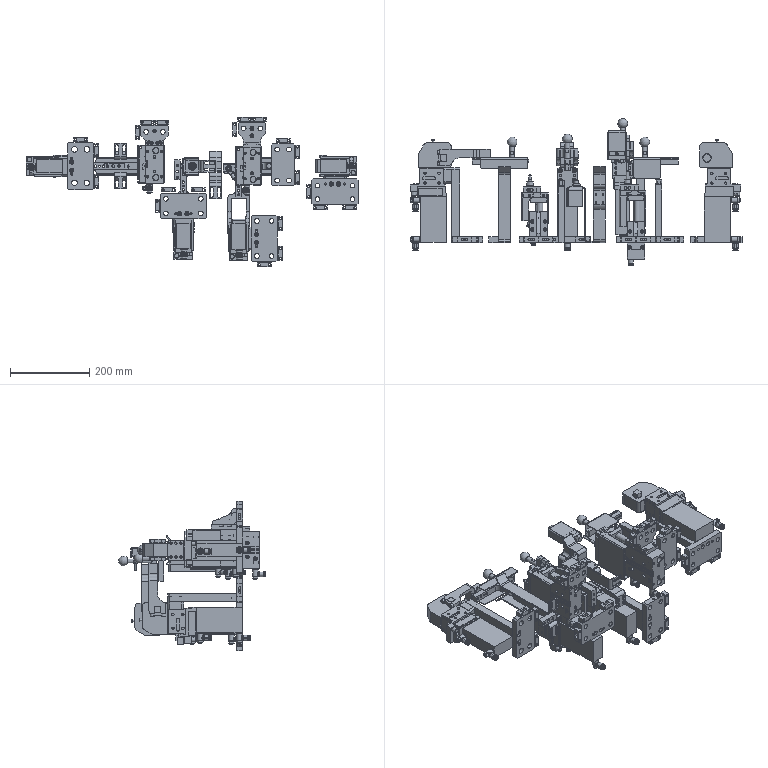Part | NX | features BREP 69 | 145 solids | 4642 faces | volume 5899459 mm3 | plane 2383 | cylinder 1566 | cone 588 | torus 65 | sphere 22 | spline 18 | commonest cylinder face diameters 6 x251 7 x91 4.917 x84 20 x73 10 x68 5 x64